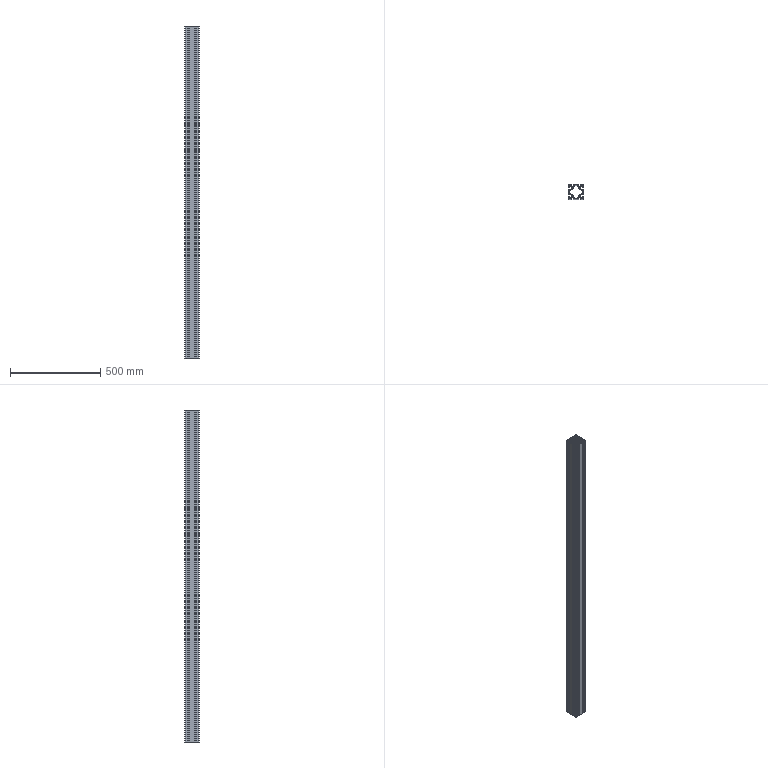Part | SolidWorks | features BaseBody 1 | 1 solid | 236 faces | box 80 x 80 x 1840 mm | volume 3133723 mm3 | plane 154 | cylinder 82 | commonest cylinder face diameters 2 x36 0.6 x20 6.8 x12 12 x10 6 x4